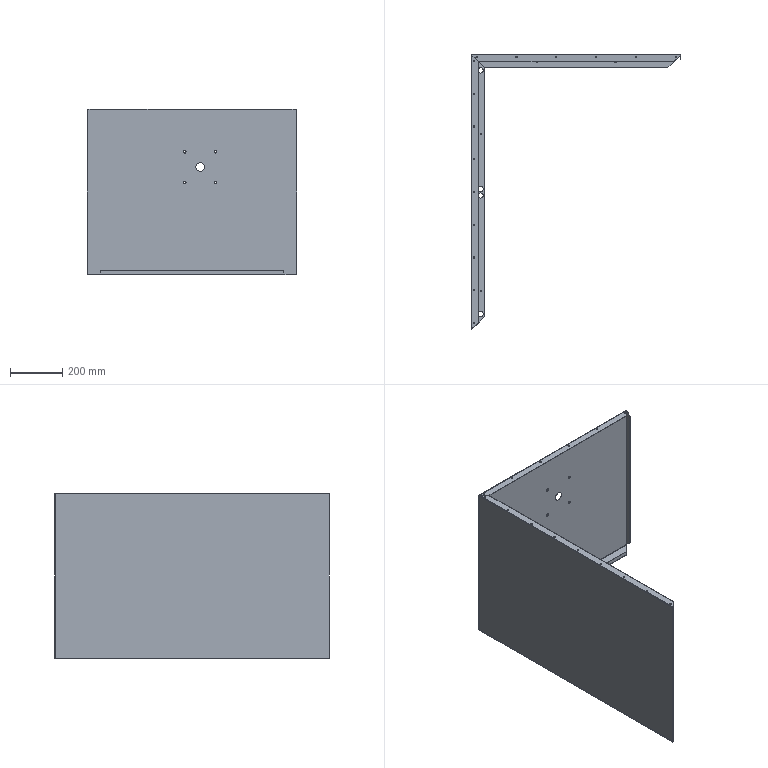Part | STEP file | HESS-408-70-15W-W-1-outer case side panel 1 | 1 solid | 134 faces | box 798.5 x 1049 x 630 mm | volume 1988997 mm3 | cylinder 72 | plane 56 | spline 6 | commonest cylinder face diameters 5 x30 0.2 x8 3.2 x8 4.2 x8 10 x8 20 x8